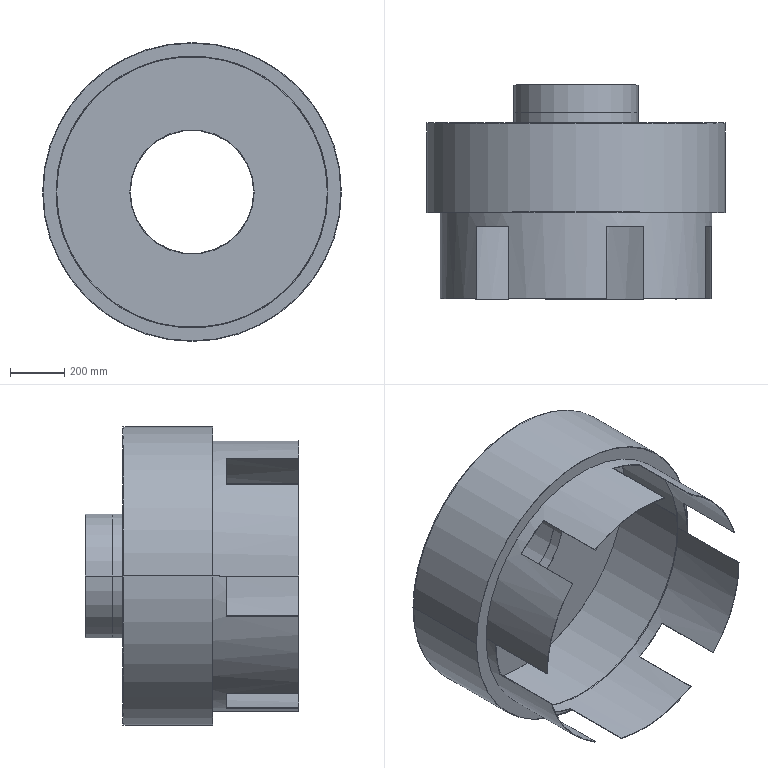Part | SolidWorks | features ICE 2, CirPattern 1, Revolution 1, Shell 1, WeldmentFeature 1 | 1 solid | 44 faces | box 1104 x 790 x 1104 mm | volume 5979369 mm3 | plane 30 | cylinder 14 | commonest cylinder face diameters 456 x2 458 x2 460 x2 1000 x2 1004 x2 1100 x2
STEP:
#1=CARTESIAN_POINT('',(229.,689.,0.));
#2=VERTEX_POINT('',#1);
#3=CARTESIAN_POINT('',(-229.,689.,0.));
#4=VERTEX_POINT('',#3);
#5=CARTESIAN_POINT('',(0.,689.,0.));
#6=DIRECTION('',(0.,1.,0.));
#7=DIRECTION('',(-1.,0.,0.));
#8=AXIS2_PLACEMENT_3D('',#5,#6,#7);
#9=CIRCLE('',#8,229.);
#10=EDGE_CURVE('',#2,#4,#9,.T.);
#11=ORIENTED_EDGE('',*,*,#10,.F.);
#12=CARTESIAN_POINT('',(229.,790.,0.));
#13=VERTEX_POINT('',#12);
#14=CARTESIAN_POINT('',(229.,689.,0.));
#15=DIRECTION('',(0.,1.,0.));
#16=VECTOR('',#15,1000.);
#17=LINE('',#14,#16);
#18=EDGE_CURVE('',#2,#13,#17,.T.);
#19=ORIENTED_EDGE('',*,*,#18,.T.);
#20=CARTESIAN_POINT('',(-229.,790.,0.));
#21=VERTEX_POINT('',#20);
#22=CARTESIAN_POINT('',(0.,790.,0.));
#23=DIRECTION('',(0.,1.,0.));
#24=DIRECTION('',(-1.,0.,0.));
#25=AXIS2_PLACEMENT_3D('',#22,#23,#24);
#26=CIRCLE('',#25,229.);
#27=EDGE_CURVE('',#13,#21,#26,.T.);
#28=ORIENTED_EDGE('',*,*,#27,.T.);
#29=CARTESIAN_POINT('',(-229.,689.,0.));
#30=DIRECTION('',(0.,1.,0.));
#31=VECTOR('',#30,1000.);
#32=LINE('',#29,#31);
#33=EDGE_CURVE('',#4,#21,#32,.T.);
#34=ORIENTED_EDGE('',*,*,#33,.F.);
#35=EDGE_LOOP('',(#11,#19,#28,#34));
#36=FACE_OUTER_BOUND('',#35,.T.);
#37=CARTESIAN_POINT('',(0.,689.,0.));
#38=DIRECTION('',(0.,1.,0.));
#39=DIRECTION('',(-1.,0.,0.));
#40=AXIS2_PLACEMENT_3D('',#37,#38,#39);
#41=CYLINDRICAL_SURFACE('',#40,229.);
#42=ADVANCED_FACE('',(#36),#41,.F.);
#43=CARTESIAN_POINT('',(-550.,648.,0.));
#44=VERTEX_POINT('',#43);
#45=CARTESIAN_POINT('',(550.,648.,0.));
#46=VERTEX_POINT('',#45);
#47=CARTESIAN_POINT('',(0.,648.,0.));
#48=DIRECTION('',(0.,-1.,0.));
#49=DIRECTION('',(-1.,0.,0.));
#50=AXIS2_PLACEMENT_3D('',#47,#48,#49);
#51=CIRCLE('',#50,550.);
#52=EDGE_CURVE('',#44,#46,#51,.T.);
#53=ORIENTED_EDGE('',*,*,#52,.F.);
#54=CARTESIAN_POINT('',(-550.,320.,0.));
#55=VERTEX_POINT('',#54);
#56=CARTESIAN_POINT('',(-550.,0.,0.));
#57=DIRECTION('',(0.,-1.,0.));
#58=VECTOR('',#57,1000.);
#59=LINE('',#56,#58);
#60=EDGE_CURVE('',#44,#55,#59,.T.);
#61=ORIENTED_EDGE('',*,*,#60,.T.);
#62=CARTESIAN_POINT('',(550.,320.,0.));
#63=VERTEX_POINT('',#62);
#64=CARTESIAN_POINT('',(0.,320.,0.));
#65=DIRECTION('',(0.,-1.,0.));
#66=DIRECTION('',(1.,0.,0.));
#67=AXIS2_PLACEMENT_3D('',#64,#65,#66);
#68=CIRCLE('',#67,550.);
#69=EDGE_CURVE('',#55,#63,#68,.T.);
#70=ORIENTED_EDGE('',*,*,#69,.T.);
#71=CARTESIAN_POINT('',(550.,0.,0.));
#72=DIRECTION('',(0.,-1.,0.));
#73=VECTOR('',#72,1000.);
#74=LINE('',#71,#73);
#75=EDGE_CURVE('',#46,#63,#74,.T.);
#76=ORIENTED_EDGE('',*,*,#75,.F.);
#77=EDGE_LOOP('',(#53,#61,#70,#76));
#78=FACE_OUTER_BOUND('',#77,.T.);
#79=CARTESIAN_POINT('',(0.,0.,0.));
#80=DIRECTION('',(0.,-1.,0.));
#81=DIRECTION('',(1.,0.,0.));
#82=AXIS2_PLACEMENT_3D('',#79,#80,#81);
#83=CYLINDRICAL_SURFACE('',#82,550.);
#84=ADVANCED_FACE('',(#78),#83,.F.);
#85=CARTESIAN_POINT('',(552.,650.,0.));
#86=VERTEX_POINT('',#85);
#87=CARTESIAN_POINT('',(-552.,650.,0.));
#88=VERTEX_POINT('',#87);
#89=CARTESIAN_POINT('',(0.,650.,0.));
#90=DIRECTION('',(0.,-1.,0.));
#91=DIRECTION('',(1.,0.,0.));
#92=AXIS2_PLACEMENT_3D('',#89,#90,#91);
#93=CIRCLE('',#92,552.);
#94=EDGE_CURVE('',#86,#88,#93,.T.);
#95=ORIENTED_EDGE('',*,*,#94,.T.);
#96=CARTESIAN_POINT('',(-552.,318.,0.));
#97=VERTEX_POINT('',#96);
#98=CARTESIAN_POINT('',(-552.,0.,0.));
#99=DIRECTION('',(0.,-1.,0.));
#100=VECTOR('',#99,1000.);
#101=LINE('',#98,#100);
#102=EDGE_CURVE('',#88,#97,#101,.T.);
#103=ORIENTED_EDGE('',*,*,#102,.T.);
#104=CARTESIAN_POINT('',(552.,318.,0.));
#105=VERTEX_POINT('',#104);
#106=CARTESIAN_POINT('',(0.,318.,0.));
#107=DIRECTION('',(0.,-1.,0.));
#108=DIRECTION('',(1.,0.,0.));
#109=AXIS2_PLACEMENT_3D('',#106,#107,#108);
#110=CIRCLE('',#109,552.);
#111=EDGE_CURVE('',#105,#97,#110,.T.);
#112=ORIENTED_EDGE('',*,*,#111,.F.);
#113=CARTESIAN_POINT('',(552.,0.,0.));
#114=DIRECTION('',(0.,-1.,0.));
#115=VECTOR('',#114,1000.);
#116=LINE('',#113,#115);
#117=EDGE_CURVE('',#86,#105,#116,.T.);
#118=ORIENTED_EDGE('',*,*,#117,.F.);
#119=EDGE_LOOP('',(#95,#103,#112,#118));
#120=FACE_OUTER_BOUND('',#119,.T.);
#121=CARTESIAN_POINT('',(0.,0.,0.));
#122=DIRECTION('',(0.,-1.,0.));
#123=DIRECTION('',(1.,0.,0.));
#124=AXIS2_PLACEMENT_3D('',#121,#122,#123);
#125=CYLINDRICAL_SURFACE('',#124,552.);
#126=ADVANCED_FACE('',(#120),#125,.T.);
#127=CARTESIAN_POINT('',(230.,790.,0.));
#128=VERTEX_POINT('',#127);
#129=CARTESIAN_POINT('',(-230.,790.,0.));
#130=VERTEX_POINT('',#129);
#131=CARTESIAN_POINT('',(0.,790.,0.));
#132=DIRECTION('',(0.,-1.,0.));
#133=DIRECTION('',(1.,0.,0.));
#134=AXIS2_PLACEMENT_3D('',#131,#132,#133);
#135=CIRCLE('',#134,230.);
#136=EDGE_CURVE('',#128,#130,#135,.T.);
#137=ORIENTED_EDGE('',*,*,#136,.T.);
#138=CARTESIAN_POINT('',(-230.,650.,0.));
#139=VERTEX_POINT('',#138);
#140=CARTESIAN_POINT('',(-230.,0.,0.));
#141=DIRECTION('',(0.,-1.,0.));
#142=VECTOR('',#141,1000.);
#143=LINE('',#140,#142);
#144=EDGE_CURVE('',#130,#139,#143,.T.);
#145=ORIENTED_EDGE('',*,*,#144,.T.);
#146=CARTESIAN_POINT('',(230.,650.,0.));
#147=VERTEX_POINT('',#146);
#148=CARTESIAN_POINT('',(0.,650.,0.));
#149=DIRECTION('',(0.,-1.,0.));
#150=DIRECTION('',(1.,0.,0.));
#151=AXIS2_PLACEMENT_3D('',#148,#149,#150);
#152=CIRCLE('',#151,230.);
#153=EDGE_CURVE('',#147,#139,#152,.T.);
#154=ORIENTED_EDGE('',*,*,#153,.F.);
#155=CARTESIAN_POINT('',(230.,0.,0.));
#156=DIRECTION('',(0.,-1.,0.));
#157=VECTOR('',#156,1000.);
#158=LINE('',#155,#157);
#159=EDGE_CURVE('',#128,#147,#158,.T.);
#160=ORIENTED_EDGE('',*,*,#159,.F.);
#161=EDGE_LOOP('',(#137,#145,#154,#160));
#162=FACE_OUTER_BOUND('',#161,.T.);
#163=CARTESIAN_POINT('',(0.,0.,0.));
#164=DIRECTION('',(0.,-1.,0.));
#165=DIRECTION('',(1.,0.,0.));
#166=AXIS2_PLACEMENT_3D('',#163,#164,#165);
#167=CYLINDRICAL_SURFACE('',#166,230.);
#168=ADVANCED_FACE('',(#162),#167,.T.);
#169=CARTESIAN_POINT('',(-228.,689.,0.));
#170=VERTEX_POINT('',#169);
#171=CARTESIAN_POINT('',(228.,689.,0.));
#172=VERTEX_POINT('',#171);
#173=CARTESIAN_POINT('',(0.,689.,0.));
#174=DIRECTION('',(0.,-1.,0.));
#175=DIRECTION('',(-1.,0.,0.));
#176=AXIS2_PLACEMENT_3D('',#173,#174,#175);
#177=CIRCLE('',#176,228.);
#178=EDGE_CURVE('',#170,#172,#177,.T.);
#179=ORIENTED_EDGE('',*,*,#178,.F.);
#180=CARTESIAN_POINT('',(-228.,648.,0.));
#181=VERTEX_POINT('',#180);
#182=CARTESIAN_POINT('',(-228.,0.,0.));
#183=DIRECTION('',(0.,-1.,0.));
#184=VECTOR('',#183,1000.);
#185=LINE('',#182,#184);
#186=EDGE_CURVE('',#170,#181,#185,.T.);
#187=ORIENTED_EDGE('',*,*,#186,.T.);
#188=CARTESIAN_POINT('',(228.,648.,0.));
#189=VERTEX_POINT('',#188);
#190=CARTESIAN_POINT('',(0.,648.,0.));
#191=DIRECTION('',(0.,-1.,0.));
#192=DIRECTION('',(-1.,0.,0.));
#193=AXIS2_PLACEMENT_3D('',#190,#191,#192);
#194=CIRCLE('',#193,228.);
#195=EDGE_CURVE('',#181,#189,#194,.T.);
#196=ORIENTED_EDGE('',*,*,#195,.T.);
#197=CARTESIAN_POINT('',(228.,0.,0.));
#198=DIRECTION('',(0.,-1.,0.));
#199=VECTOR('',#198,1000.);
#200=LINE('',#197,#199);
#201=EDGE_CURVE('',#172,#189,#200,.T.);
#202=ORIENTED_EDGE('',*,*,#201,.F.);
#203=EDGE_LOOP('',(#179,#187,#196,#202));
#204=FACE_OUTER_BOUND('',#203,.T.);
#205=CARTESIAN_POINT('',(0.,0.,0.));
#206=DIRECTION('',(0.,-1.,0.));
#207=DIRECTION('',(1.,0.,0.));
#208=AXIS2_PLACEMENT_3D('',#205,#206,#207);
#209=CYLINDRICAL_SURFACE('',#208,228.);
#210=ADVANCED_FACE('',(#204),#209,.F.);
#211=CARTESIAN_POINT('',(-500.,320.,0.));
#212=VERTEX_POINT('',#211);
#213=CARTESIAN_POINT('',(500.,320.,0.));
#214=VERTEX_POINT('',#213);
#215=CARTESIAN_POINT('',(0.,320.,0.));
#216=DIRECTION('',(0.,-1.,0.));
#217=DIRECTION('',(1.,0.,0.));
#218=AXIS2_PLACEMENT_3D('',#215,#216,#217);
#219=CIRCLE('',#218,500.);
#220=EDGE_CURVE('',#212,#214,#219,.T.);
#221=ORIENTED_EDGE('',*,*,#220,.F.);
#222=CARTESIAN_POINT('',(-500.,268.,0.));
#223=VERTEX_POINT('',#222);
#224=CARTESIAN_POINT('',(-500.,0.,0.));
#225=DIRECTION('',(0.,-1.,0.));
#226=VECTOR('',#225,1000.);
#227=LINE('',#224,#226);
#228=EDGE_CURVE('',#212,#223,#227,.T.);
#229=ORIENTED_EDGE('',*,*,#228,.T.);
#230=CARTESIAN_POINT('',(-477.679,268.,-147.726));
#231=VERTEX_POINT('',#230);
#232=CARTESIAN_POINT('',(0.,268.,0.));
#233=DIRECTION('',(0.,1.,0.));
#234=DIRECTION('',(1.,0.,0.));
#235=AXIS2_PLACEMENT_3D('',#232,#233,#234);
#236=CIRCLE('',#235,500.);
#237=EDGE_CURVE('',#231,#223,#236,.T.);
#238=ORIENTED_EDGE('',*,*,#237,.F.);
#239=CARTESIAN_POINT('',(-477.679,0.,-147.726));
#240=VERTEX_POINT('',#239);
#241=CARTESIAN_POINT('',(-477.679,0.,-147.726));
#242=DIRECTION('',(0.,1.,0.));
#243=VECTOR('',#242,1000.);
#244=LINE('',#241,#243);
#245=EDGE_CURVE('',#240,#231,#244,.T.);
#246=ORIENTED_EDGE('',*,*,#245,.F.);
#247=CARTESIAN_POINT('',(-250.,0.,-433.013));
#248=VERTEX_POINT('',#247);
#249=CARTESIAN_POINT('',(0.,0.,0.));
#250=DIRECTION('',(0.,-1.,0.));
#251=DIRECTION('',(1.,0.,0.));
#252=AXIS2_PLACEMENT_3D('',#249,#250,#251);
#253=CIRCLE('',#252,500.);
#254=EDGE_CURVE('',#240,#248,#253,.T.);
#255=ORIENTED_EDGE('',*,*,#254,.T.);
#256=CARTESIAN_POINT('',(-250.,268.,-433.013));
#257=VERTEX_POINT('',#256);
#258=CARTESIAN_POINT('',(-250.,0.,-433.013));
#259=DIRECTION('',(0.,-1.,0.));
#260=VECTOR('',#259,1000.);
#261=LINE('',#258,#260);
#262=EDGE_CURVE('',#257,#248,#261,.T.);
#263=ORIENTED_EDGE('',*,*,#262,.F.);
#264=CARTESIAN_POINT('',(-110.905,268.,-487.545));
#265=VERTEX_POINT('',#264);
#266=CARTESIAN_POINT('',(0.,268.,0.));
#267=DIRECTION('',(0.,1.,0.));
#268=DIRECTION('',(1.,0.,0.));
#269=AXIS2_PLACEMENT_3D('',#266,#267,#268);
#270=CIRCLE('',#269,500.);
#271=EDGE_CURVE('',#265,#257,#270,.T.);
#272=ORIENTED_EDGE('',*,*,#271,.F.);
#273=CARTESIAN_POINT('',(-110.905,0.,-487.545));
#274=VERTEX_POINT('',#273);
#275=CARTESIAN_POINT('',(-110.905,0.,-487.545));
#276=DIRECTION('',(0.,1.,0.));
#277=VECTOR('',#276,1000.);
#278=LINE('',#275,#277);
#279=EDGE_CURVE('',#274,#265,#278,.T.);
#280=ORIENTED_EDGE('',*,*,#279,.F.);
#281=CARTESIAN_POINT('',(250.,0.,-433.013));
#282=VERTEX_POINT('',#281);
#283=CARTESIAN_POINT('',(0.,0.,0.));
#284=DIRECTION('',(0.,-1.,0.));
#285=DIRECTION('',(1.,0.,0.));
#286=AXIS2_PLACEMENT_3D('',#283,#284,#285);
#287=CIRCLE('',#286,500.);
#288=EDGE_CURVE('',#274,#282,#287,.T.);
#289=ORIENTED_EDGE('',*,*,#288,.T.);
#290=CARTESIAN_POINT('',(250.,268.,-433.013));
#291=VERTEX_POINT('',#290);
#292=CARTESIAN_POINT('',(250.,0.,-433.013));
#293=DIRECTION('',(0.,-1.,0.));
#294=VECTOR('',#293,1000.);
#295=LINE('',#292,#294);
#296=EDGE_CURVE('',#291,#282,#295,.T.);
#297=ORIENTED_EDGE('',*,*,#296,.F.);
#298=CARTESIAN_POINT('',(366.774,268.,-339.819));
#299=VERTEX_POINT('',#298);
#300=CARTESIAN_POINT('',(0.,268.,0.));
#301=DIRECTION('',(0.,1.,0.));
#302=DIRECTION('',(1.,0.,0.));
#303=AXIS2_PLACEMENT_3D('',#300,#301,#302);
#304=CIRCLE('',#303,500.);
#305=EDGE_CURVE('',#299,#291,#304,.T.);
#306=ORIENTED_EDGE('',*,*,#305,.F.);
#307=CARTESIAN_POINT('',(366.774,0.,-339.819));
#308=VERTEX_POINT('',#307);
#309=CARTESIAN_POINT('',(366.774,0.,-339.819));
#310=DIRECTION('',(0.,1.,0.));
#311=VECTOR('',#310,1000.);
#312=LINE('',#309,#311);
#313=EDGE_CURVE('',#308,#299,#312,.T.);
#314=ORIENTED_EDGE('',*,*,#313,.F.);
#315=CARTESIAN_POINT('',(500.,0.,0.));
#316=VERTEX_POINT('',#315);
#317=CARTESIAN_POINT('',(0.,0.,0.));
#318=DIRECTION('',(0.,-1.,0.));
#319=DIRECTION('',(1.,0.,0.));
#320=AXIS2_PLACEMENT_3D('',#317,#318,#319);
#321=CIRCLE('',#320,500.);
#322=EDGE_CURVE('',#308,#316,#321,.T.);
#323=ORIENTED_EDGE('',*,*,#322,.T.);
#324=CARTESIAN_POINT('',(500.,268.,0.));
#325=VERTEX_POINT('',#324);
#326=CARTESIAN_POINT('',(500.,0.,0.));
#327=DIRECTION('',(0.,-1.,0.));
#328=VECTOR('',#327,1000.);
#329=LINE('',#326,#328);
#330=EDGE_CURVE('',#325,#316,#329,.T.);
#331=ORIENTED_EDGE('',*,*,#330,.F.);
#332=CARTESIAN_POINT('',(500.,0.,0.));
#333=DIRECTION('',(0.,-1.,0.));
#334=VECTOR('',#333,1000.);
#335=LINE('',#332,#334);
#336=EDGE_CURVE('',#214,#325,#335,.T.);
#337=ORIENTED_EDGE('',*,*,#336,.F.);
#338=EDGE_LOOP('',(#221,#229,#238,#246,#255,#263,#272,#280,#289,#297,#306,#314,#323,#331,#337));
#339=FACE_OUTER_BOUND('',#338,.T.);
#340=CARTESIAN_POINT('',(0.,0.,0.));
#341=DIRECTION('',(0.,-1.,0.));
#342=DIRECTION('',(1.,0.,0.));
#343=AXIS2_PLACEMENT_3D('',#340,#341,#342);
#344=CYLINDRICAL_SURFACE('',#343,500.);
#345=ADVANCED_FACE('',(#339),#344,.F.);
#346=CARTESIAN_POINT('',(502.,318.,0.));
#347=VERTEX_POINT('',#346);
#348=CARTESIAN_POINT('',(-502.,318.,0.));
#349=VERTEX_POINT('',#348);
#350=CARTESIAN_POINT('',(0.,318.,0.));
#351=DIRECTION('',(0.,-1.,0.));
#352=DIRECTION('',(1.,0.,0.));
#353=AXIS2_PLACEMENT_3D('',#350,#351,#352);
#354=CIRCLE('',#353,502.);
#355=EDGE_CURVE('',#347,#349,#354,.T.);
#356=ORIENTED_EDGE('',*,*,#355,.T.);
#357=CARTESIAN_POINT('',(-502.,268.,0.));
#358=VERTEX_POINT('',#357);
#359=CARTESIAN_POINT('',(-502.,0.,0.));
#360=DIRECTION('',(0.,-1.,0.));
#361=VECTOR('',#360,1000.);
#362=LINE('',#359,#361);
#363=EDGE_CURVE('',#349,#358,#362,.T.);
#364=ORIENTED_EDGE('',*,*,#363,.T.);
#365=CARTESIAN_POINT('',(-502.,0.,0.));
#366=VERTEX_POINT('',#365);
#367=CARTESIAN_POINT('',(-502.,0.,0.));
#368=DIRECTION('',(0.,-1.,0.));
#369=VECTOR('',#368,1000.);
#370=LINE('',#367,#369);
#371=EDGE_CURVE('',#358,#366,#370,.T.);
#372=ORIENTED_EDGE('',*,*,#371,.T.);
#373=CARTESIAN_POINT('',(-368.241,0.,341.179));
#374=VERTEX_POINT('',#373);
#375=CARTESIAN_POINT('',(0.,0.,0.));
#376=DIRECTION('',(0.,-1.,0.));
#377=DIRECTION('',(1.,0.,0.));
#378=AXIS2_PLACEMENT_3D('',#375,#376,#377);
#379=CIRCLE('',#378,502.);
#380=EDGE_CURVE('',#374,#366,#379,.T.);
#381=ORIENTED_EDGE('',*,*,#380,.F.);
#382=CARTESIAN_POINT('',(-368.241,268.,341.179));
#383=VERTEX_POINT('',#382);
#384=CARTESIAN_POINT('',(-368.241,0.,341.179));
#385=DIRECTION('',(0.,1.,0.));
#386=VECTOR('',#385,1000.);
#387=LINE('',#384,#386);
#388=EDGE_CURVE('',#374,#383,#387,.T.);
#389=ORIENTED_EDGE('',*,*,#388,.T.);
#390=CARTESIAN_POINT('',(-251.,268.,434.745));
#391=VERTEX_POINT('',#390);
#392=CARTESIAN_POINT('',(0.,268.,0.));
#393=DIRECTION('',(0.,1.,0.));
#394=DIRECTION('',(1.,0.,0.));
#395=AXIS2_PLACEMENT_3D('',#392,#393,#394);
#396=CIRCLE('',#395,502.);
#397=EDGE_CURVE('',#383,#391,#396,.T.);
#398=ORIENTED_EDGE('',*,*,#397,.T.);
#399=CARTESIAN_POINT('',(-251.,0.,434.745));
#400=VERTEX_POINT('',#399);
#401=CARTESIAN_POINT('',(-251.,0.,434.745));
#402=DIRECTION('',(0.,-1.,0.));
#403=VECTOR('',#402,1000.);
#404=LINE('',#401,#403);
#405=EDGE_CURVE('',#391,#400,#404,.T.);
#406=ORIENTED_EDGE('',*,*,#405,.T.);
#407=CARTESIAN_POINT('',(111.349,0.,489.495));
#408=VERTEX_POINT('',#407);
#409=CARTESIAN_POINT('',(0.,0.,0.));
#410=DIRECTION('',(0.,-1.,0.));
#411=DIRECTION('',(1.,0.,0.));
#412=AXIS2_PLACEMENT_3D('',#409,#410,#411);
#413=CIRCLE('',#412,502.);
#414=EDGE_CURVE('',#408,#400,#413,.T.);
#415=ORIENTED_EDGE('',*,*,#414,.F.);
#416=CARTESIAN_POINT('',(111.349,268.,489.495));
#417=VERTEX_POINT('',#416);
#418=CARTESIAN_POINT('',(111.349,0.,489.495));
#419=DIRECTION('',(0.,1.,0.));
#420=VECTOR('',#419,1000.);
#421=LINE('',#418,#420);
#422=EDGE_CURVE('',#408,#417,#421,.T.);
#423=ORIENTED_EDGE('',*,*,#422,.T.);
#424=CARTESIAN_POINT('',(251.,268.,434.745));
#425=VERTEX_POINT('',#424);
#426=CARTESIAN_POINT('',(0.,268.,0.));
#427=DIRECTION('',(0.,1.,0.));
#428=DIRECTION('',(1.,0.,0.));
#429=AXIS2_PLACEMENT_3D('',#426,#427,#428);
#430=CIRCLE('',#429,502.);
#431=EDGE_CURVE('',#417,#425,#430,.T.);
#432=ORIENTED_EDGE('',*,*,#431,.T.);
#433=CARTESIAN_POINT('',(251.,0.,434.745));
#434=VERTEX_POINT('',#433);
#435=CARTESIAN_POINT('',(251.,0.,434.745));
#436=DIRECTION('',(0.,-1.,0.));
#437=VECTOR('',#436,1000.);
#438=LINE('',#435,#437);
#439=EDGE_CURVE('',#425,#434,#438,.T.);
#440=ORIENTED_EDGE('',*,*,#439,.T.);
#441=CARTESIAN_POINT('',(479.59,0.,148.316));
#442=VERTEX_POINT('',#441);
#443=CARTESIAN_POINT('',(0.,0.,0.));
#444=DIRECTION('',(0.,-1.,0.));
#445=DIRECTION('',(1.,0.,0.));
#446=AXIS2_PLACEMENT_3D('',#443,#444,#445);
#447=CIRCLE('',#446,502.);
#448=EDGE_CURVE('',#442,#434,#447,.T.);
#449=ORIENTED_EDGE('',*,*,#448,.F.);
#450=CARTESIAN_POINT('',(479.59,268.,148.316));
#451=VERTEX_POINT('',#450);
#452=CARTESIAN_POINT('',(479.59,0.,148.316));
#453=DIRECTION('',(0.,1.,0.));
#454=VECTOR('',#453,1000.);
#455=LINE('',#452,#454);
#456=EDGE_CURVE('',#442,#451,#455,.T.);
#457=ORIENTED_EDGE('',*,*,#456,.T.);
#458=CARTESIAN_POINT('',(502.,268.,0.));
#459=VERTEX_POINT('',#458);
#460=CARTESIAN_POINT('',(0.,268.,0.));
#461=DIRECTION('',(0.,1.,0.));
#462=DIRECTION('',(1.,0.,0.));
#463=AXIS2_PLACEMENT_3D('',#460,#461,#462);
#464=CIRCLE('',#463,502.);
#465=EDGE_CURVE('',#451,#459,#464,.T.);
#466=ORIENTED_EDGE('',*,*,#465,.T.);
#467=CARTESIAN_POINT('',(502.,0.,0.));
#468=DIRECTION('',(0.,-1.,0.));
#469=VECTOR('',#468,1000.);
#470=LINE('',#467,#469);
#471=EDGE_CURVE('',#347,#459,#470,.T.);
#472=ORIENTED_EDGE('',*,*,#471,.F.);
#473=EDGE_LOOP('',(#356,#364,#372,#381,#389,#398,#406,#415,#423,#432,#440,#449,#457,#466,#472));
#474=FACE_OUTER_BOUND('',#473,.T.);
#475=CARTESIAN_POINT('',(0.,0.,0.));
#476=DIRECTION('',(0.,-1.,0.));
#477=DIRECTION('',(1.,0.,0.));
#478=AXIS2_PLACEMENT_3D('',#475,#476,#477);
#479=CYLINDRICAL_SURFACE('',#478,502.);
#480=ADVANCED_FACE('',(#474),#479,.T.);
#481=ORIENTED_EDGE('',*,*,#448,.T.);
#482=CARTESIAN_POINT('',(250.,0.,433.013));
#483=VERTEX_POINT('',#482);
#484=CARTESIAN_POINT('',(0.,0.,0.));
#485=DIRECTION('',(-0.5,0.,-0.866));
#486=VECTOR('',#485,1000.);
#487=LINE('',#484,#486);
#488=EDGE_CURVE('',#434,#483,#487,.T.);
#489=ORIENTED_EDGE('',*,*,#488,.T.);
#490=CARTESIAN_POINT('',(477.679,0.,147.726));
#491=VERTEX_POINT('',#490);
#492=CARTESIAN_POINT('',(0.,0.,0.));
#493=DIRECTION('',(0.,-1.,0.));
#494=DIRECTION('',(1.,0.,0.));
#495=AXIS2_PLACEMENT_3D('',#492,#493,#494);
#496=CIRCLE('',#495,500.);
#497=EDGE_CURVE('',#491,#483,#496,.T.);
#498=ORIENTED_EDGE('',*,*,#497,.F.);
#499=CARTESIAN_POINT('',(0.,0.,0.));
#500=DIRECTION('',(0.9554,0.,0.2955));
#501=VECTOR('',#500,1000.);
#502=LINE('',#499,#501);
#503=EDGE_CURVE('',#491,#442,#502,.T.);
#504=ORIENTED_EDGE('',*,*,#503,.T.);
#505=EDGE_LOOP('',(#481,#489,#498,#504));
#506=FACE_OUTER_BOUND('',#505,.T.);
#507=CARTESIAN_POINT('',(502.,0.,0.));
#508=DIRECTION('',(0.,-1.,0.));
#509=DIRECTION('',(1.,0.,0.));
#510=AXIS2_PLACEMENT_3D('',#507,#508,#509);
#511=PLANE('',#510);
#512=ADVANCED_FACE('',(#506),#511,.T.);
#513=CARTESIAN_POINT('',(110.905,0.,487.545));
#514=VERTEX_POINT('',#513);
#515=CARTESIAN_POINT('',(-250.,0.,433.013));
#516=VERTEX_POINT('',#515);
#517=CARTESIAN_POINT('',(0.,0.,0.));
#518=DIRECTION('',(0.,-1.,0.));
#519=DIRECTION('',(1.,0.,0.));
#520=AXIS2_PLACEMENT_3D('',#517,#518,#519);
#521=CIRCLE('',#520,500.);
#522=EDGE_CURVE('',#514,#516,#521,.T.);
#523=ORIENTED_EDGE('',*,*,#522,.F.);
#524=CARTESIAN_POINT('',(0.,0.,0.));
#525=DIRECTION('',(0.2218,0.,0.9751));
#526=VECTOR('',#525,1000.);
#527=LINE('',#524,#526);
#528=EDGE_CURVE('',#514,#408,#527,.T.);
#529=ORIENTED_EDGE('',*,*,#528,.T.);
#530=ORIENTED_EDGE('',*,*,#414,.T.);
#531=CARTESIAN_POINT('',(0.,0.,0.));
#532=DIRECTION('',(0.5,0.,-0.866));
#533=VECTOR('',#532,1000.);
#534=LINE('',#531,#533);
#535=EDGE_CURVE('',#400,#516,#534,.T.);
#536=ORIENTED_EDGE('',*,*,#535,.T.);
#537=EDGE_LOOP('',(#523,#529,#530,#536));
#538=FACE_OUTER_BOUND('',#537,.T.);
#539=CARTESIAN_POINT('',(502.,0.,0.));
#540=DIRECTION('',(0.,-1.,0.));
#541=DIRECTION('',(1.,0.,0.));
#542=AXIS2_PLACEMENT_3D('',#539,#540,#541);
#543=PLANE('',#542);
#544=ADVANCED_FACE('',(#538),#543,.T.);
#545=ORIENTED_EDGE('',*,*,#363,.F.);
#546=CARTESIAN_POINT('',(0.,318.,0.));
#547=DIRECTION('',(0.,-1.,0.));
#548=DIRECTION('',(1.,0.,0.));
#549=AXIS2_PLACEMENT_3D('',#546,#547,#548);
#550=CIRCLE('',#549,502.);
#551=EDGE_CURVE('',#349,#347,#550,.T.);
#552=ORIENTED_EDGE('',*,*,#551,.T.);
#553=ORIENTED_EDGE('',*,*,#471,.T.);
#554=CARTESIAN_POINT('',(502.,0.,0.));
#555=VERTEX_POINT('',#554);
#556=CARTESIAN_POINT('',(502.,0.,0.));
#557=DIRECTION('',(0.,-1.,0.));
#558=VECTOR('',#557,1000.);
#559=LINE('',#556,#558);
#560=EDGE_CURVE('',#459,#555,#559,.T.);
#561=ORIENTED_EDGE('',*,*,#560,.T.);
#562=CARTESIAN_POINT('',(368.241,0.,-341.179));
#563=VERTEX_POINT('',#562);
#564=CARTESIAN_POINT('',(0.,0.,0.));
#565=DIRECTION('',(0.,-1.,0.));
#566=DIRECTION('',(1.,0.,0.));
#567=AXIS2_PLACEMENT_3D('',#564,#565,#566);
#568=CIRCLE('',#567,502.);
#569=EDGE_CURVE('',#563,#555,#568,.T.);
#570=ORIENTED_EDGE('',*,*,#569,.F.);
#571=CARTESIAN_POINT('',(368.241,268.,-341.179));
#572=VERTEX_POINT('',#571);
#573=CARTESIAN_POINT('',(368.241,0.,-341.179));
#574=DIRECTION('',(0.,1.,0.));
#575=VECTOR('',#574,1000.);
#576=LINE('',#573,#575);
#577=EDGE_CURVE('',#563,#572,#576,.T.);
#578=ORIENTED_EDGE('',*,*,#577,.T.);
#579=CARTESIAN_POINT('',(251.,268.,-434.745));
#580=VERTEX_POINT('',#579);
#581=CARTESIAN_POINT('',(0.,268.,0.));
#582=DIRECTION('',(0.,1.,0.));
#583=DIRECTION('',(1.,0.,0.));
#584=AXIS2_PLACEMENT_3D('',#581,#582,#583);
#585=CIRCLE('',#584,502.);
#586=EDGE_CURVE('',#572,#580,#585,.T.);
#587=ORIENTED_EDGE('',*,*,#586,.T.);
#588=CARTESIAN_POINT('',(251.,0.,-434.745));
#589=VERTEX_POINT('',#588);
#590=CARTESIAN_POINT('',(251.,0.,-434.745));
#591=DIRECTION('',(0.,-1.,0.));
#592=VECTOR('',#591,1000.);
#593=LINE('',#590,#592);
#594=EDGE_CURVE('',#580,#589,#593,.T.);
#595=ORIENTED_EDGE('',*,*,#594,.T.);
#596=CARTESIAN_POINT('',(-111.349,0.,-489.495));
#597=VERTEX_POINT('',#596);
#598=CARTESIAN_POINT('',(0.,0.,0.));
#599=DIRECTION('',(0.,-1.,0.));
#600=DIRECTION('',(1.,0.,0.));
#601=AXIS2_PLACEMENT_3D('',#598,#599,#600);
#602=CIRCLE('',#601,502.);
#603=EDGE_CURVE('',#597,#589,#602,.T.);
#604=ORIENTED_EDGE('',*,*,#603,.F.);
#605=CARTESIAN_POINT('',(-111.349,268.,-489.495));
#606=VERTEX_POINT('',#605);
#607=CARTESIAN_POINT('',(-111.349,0.,-489.495));
#608=DIRECTION('',(0.,1.,0.));
#609=VECTOR('',#608,1000.);
#610=LINE('',#607,#609);
#611=EDGE_CURVE('',#597,#606,#610,.T.);
#612=ORIENTED_EDGE('',*,*,#611,.T.);
#613=CARTESIAN_POINT('',(-251.,268.,-434.745));
#614=VERTEX_POINT('',#613);
#615=CARTESIAN_POINT('',(0.,268.,0.));
#616=DIRECTION('',(0.,1.,0.));
#617=DIRECTION('',(1.,0.,0.));
#618=AXIS2_PLACEMENT_3D('',#615,#616,#617);
#619=CIRCLE('',#618,502.);
#620=EDGE_CURVE('',#606,#614,#619,.T.);
#621=ORIENTED_EDGE('',*,*,#620,.T.);
#622=CARTESIAN_POINT('',(-251.,0.,-434.745));
#623=VERTEX_POINT('',#622);
#624=CARTESIAN_POINT('',(-251.,0.,-434.745));
#625=DIRECTION('',(0.,-1.,0.));
#626=VECTOR('',#625,1000.);
#627=LINE('',#624,#626);
#628=EDGE_CURVE('',#614,#623,#627,.T.);
#629=ORIENTED_EDGE('',*,*,#628,.T.);
#630=CARTESIAN_POINT('',(-479.59,0.,-148.316));
#631=VERTEX_POINT('',#630);
#632=CARTESIAN_POINT('',(0.,0.,0.));
#633=DIRECTION('',(0.,-1.,0.));
#634=DIRECTION('',(1.,0.,0.));
#635=AXIS2_PLACEMENT_3D('',#632,#633,#634);
#636=CIRCLE('',#635,502.);
#637=EDGE_CURVE('',#631,#623,#636,.T.);
#638=ORIENTED_EDGE('',*,*,#637,.F.);
#639=CARTESIAN_POINT('',(-479.59,268.,-148.316));
#640=VERTEX_POINT('',#639);
#641=CARTESIAN_POINT('',(-479.59,0.,-148.316));
#642=DIRECTION('',(0.,1.,0.));
#643=VECTOR('',#642,1000.);
#644=LINE('',#641,#643);
#645=EDGE_CURVE('',#631,#640,#644,.T.);
#646=ORIENTED_EDGE('',*,*,#645,.T.);
#647=CARTESIAN_POINT('',(0.,268.,0.));
#648=DIRECTION('',(0.,1.,0.));
#649=DIRECTION('',(1.,0.,0.));
#650=AXIS2_PLACEMENT_3D('',#647,#648,#649);
#651=CIRCLE('',#650,502.);
#652=EDGE_CURVE('',#640,#358,#651,.T.);
#653=ORIENTED_EDGE('',*,*,#652,.T.);
#654=EDGE_LOOP('',(#545,#552,#553,#561,#570,#578,#587,#595,#604,#612,#621,#629,#638,#646,#653));
#655=FACE_OUTER_BOUND('',#654,.T.);
#656=CARTESIAN_POINT('',(0.,0.,0.));
#657=DIRECTION('',(0.,-1.,0.));
#658=DIRECTION('',(1.,0.,0.));
#659=AXIS2_PLACEMENT_3D('',#656,#657,#658);
#660=CYLINDRICAL_SURFACE('',#659,502.);
#661=ADVANCED_FACE('',(#655),#660,.T.);
#662=ORIENTED_EDGE('',*,*,#228,.F.);
#663=CARTESIAN_POINT('',(0.,320.,0.));
#664=DIRECTION('',(0.,-1.,0.));
#665=DIRECTION('',(1.,0.,0.));
#666=AXIS2_PLACEMENT_3D('',#663,#664,#665);
#667=CIRCLE('',#666,500.);
#668=EDGE_CURVE('',#214,#212,#667,.T.);
#669=ORIENTED_EDGE('',*,*,#668,.F.);
#670=ORIENTED_EDGE('',*,*,#336,.T.);
#671=CARTESIAN_POINT('',(477.679,268.,147.726));
#672=VERTEX_POINT('',#671);
#673=CARTESIAN_POINT('',(0.,268.,0.));
#674=DIRECTION('',(0.,1.,0.));
#675=DIRECTION('',(1.,0.,0.));
#676=AXIS2_PLACEMENT_3D('',#673,#674,#675);
#677=CIRCLE('',#676,500.);
#678=EDGE_CURVE('',#672,#325,#677,.T.);
#679=ORIENTED_EDGE('',*,*,#678,.F.);
#680=CARTESIAN_POINT('',(477.679,0.,147.726));
#681=DIRECTION('',(0.,1.,0.));
#682=VECTOR('',#681,1000.);
#683=LINE('',#680,#682);
#684=EDGE_CURVE('',#491,#672,#683,.T.);
#685=ORIENTED_EDGE('',*,*,#684,.F.);
#686=ORIENTED_EDGE('',*,*,#497,.T.);
#687=CARTESIAN_POINT('',(250.,268.,433.013));
#688=VERTEX_POINT('',#687);
#689=CARTESIAN_POINT('',(250.,0.,433.013));
#690=DIRECTION('',(0.,-1.,0.));
#691=VECTOR('',#690,1000.);
#692=LINE('',#689,#691);
#693=EDGE_CURVE('',#688,#483,#692,.T.);
#694=ORIENTED_EDGE('',*,*,#693,.F.);
#695=CARTESIAN_POINT('',(110.905,268.,487.545));
#696=VERTEX_POINT('',#695);
#697=CARTESIAN_POINT('',(0.,268.,0.));
#698=DIRECTION('',(0.,1.,0.));
#699=DIRECTION('',(1.,0.,0.));
#700=AXIS2_PLACEMENT_3D('',#697,#698,#699);
#701=CIRCLE('',#700,500.);
#702=EDGE_CURVE('',#696,#688,#701,.T.);
#703=ORIENTED_EDGE('',*,*,#702,.F.);
#704=CARTESIAN_POINT('',(110.905,0.,487.545));
#705=DIRECTION('',(0.,1.,0.));
#706=VECTOR('',#705,1000.);
#707=LINE('',#704,#706);
#708=EDGE_CURVE('',#514,#696,#707,.T.);
#709=ORIENTED_EDGE('',*,*,#708,.F.);
#710=ORIENTED_EDGE('',*,*,#522,.T.);
#711=CARTESIAN_POINT('',(-250.,268.,433.013));
#712=VERTEX_POINT('',#711);
#713=CARTESIAN_POINT('',(-250.,0.,433.013));
#714=DIRECTION('',(0.,-1.,0.));
#715=VECTOR('',#714,1000.);
#716=LINE('',#713,#715);
#717=EDGE_CURVE('',#712,#516,#716,.T.);
#718=ORIENTED_EDGE('',*,*,#717,.F.);
#719=CARTESIAN_POINT('',(-366.774,268.,339.819));
#720=VERTEX_POINT('',#719);
#721=CARTESIAN_POINT('',(0.,268.,0.));
#722=DIRECTION('',(0.,1.,0.));
#723=DIRECTION('',(1.,0.,0.));
#724=AXIS2_PLACEMENT_3D('',#721,#722,#723);
#725=CIRCLE('',#724,500.);
#726=EDGE_CURVE('',#720,#712,#725,.T.);
#727=ORIENTED_EDGE('',*,*,#726,.F.);
#728=CARTESIAN_POINT('',(-366.774,0.,339.819));
#729=VERTEX_POINT('',#728);
#730=CARTESIAN_POINT('',(-366.774,0.,339.819));
#731=DIRECTION('',(0.,1.,0.));
#732=VECTOR('',#731,1000.);
#733=LINE('',#730,#732);
#734=EDGE_CURVE('',#729,#720,#733,.T.);
#735=ORIENTED_EDGE('',*,*,#734,.F.);
#736=CARTESIAN_POINT('',(-500.,0.,0.));
#737=VERTEX_POINT('',#736);
#738=CARTESIAN_POINT('',(0.,0.,0.));
#739=DIRECTION('',(0.,-1.,0.));
#740=DIRECTION('',(1.,0.,0.));
#741=AXIS2_PLACEMENT_3D('',#738,#739,#740);
#742=CIRCLE('',#741,500.);
#743=EDGE_CURVE('',#729,#737,#742,.T.);
#744=ORIENTED_EDGE('',*,*,#743,.T.);
#745=CARTESIAN_POINT('',(-500.,0.,0.));
#746=DIRECTION('',(0.,-1.,0.));
#747=VECTOR('',#746,1000.);
#748=LINE('',#745,#747);
#749=EDGE_CURVE('',#223,#737,#748,.T.);
#750=ORIENTED_EDGE('',*,*,#749,.F.);
#751=EDGE_LOOP('',(#662,#669,#670,#679,#685,#686,#694,#703,#709,#710,#718,#727,#735,#744,#750));
#752=FACE_OUTER_BOUND('',#751,.T.);
#753=CARTESIAN_POINT('',(0.,0.,0.));
#754=DIRECTION('',(0.,-1.,0.));
#755=DIRECTION('',(1.,0.,0.));
#756=AXIS2_PLACEMENT_3D('',#753,#754,#755);
#757=CYLINDRICAL_SURFACE('',#756,500.);
#758=ADVANCED_FACE('',(#752),#757,.F.);
#759=ORIENTED_EDGE('',*,*,#743,.F.);
#760=CARTESIAN_POINT('',(0.,0.,0.));
#761=DIRECTION('',(-0.7335,0.,0.6796));
#762=VECTOR('',#761,1000.);
#763=LINE('',#760,#762);
#764=EDGE_CURVE('',#729,#374,#763,.T.);
#765=ORIENTED_EDGE('',*,*,#764,.T.);
#766=ORIENTED_EDGE('',*,*,#380,.T.);
#767=CARTESIAN_POINT('',(0.,0.,0.));
#768=DIRECTION('',(1.,0.,0.));
#769=VECTOR('',#768,1000.);
#770=LINE('',#767,#769);
#771=EDGE_CURVE('',#366,#737,#770,.T.);
#772=ORIENTED_EDGE('',*,*,#771,.T.);
#773=EDGE_LOOP('',(#759,#765,#766,#772));
#774=FACE_OUTER_BOUND('',#773,.T.);
#775=CARTESIAN_POINT('',(502.,0.,0.));
#776=DIRECTION('',(0.,-1.,0.));
#777=DIRECTION('',(1.,0.,0.));
#778=AXIS2_PLACEMENT_3D('',#775,#776,#777);
#779=PLANE('',#778);
#780=ADVANCED_FACE('',(#774),#779,.T.);
#781=ORIENTED_EDGE('',*,*,#254,.F.);
#782=CARTESIAN_POINT('',(0.,0.,0.));
#783=DIRECTION('',(-0.9554,0.,-0.2955));
#784=VECTOR('',#783,1000.);
#785=LINE('',#782,#784);
#786=EDGE_CURVE('',#240,#631,#785,.T.);
#787=ORIENTED_EDGE('',*,*,#786,.T.);
#788=ORIENTED_EDGE('',*,*,#637,.T.);
#789=CARTESIAN_POINT('',(0.,0.,0.));
#790=DIRECTION('',(0.5,0.,0.866));
#791=VECTOR('',#790,1000.);
#792=LINE('',#789,#791);
#793=EDGE_CURVE('',#623,#248,#792,.T.);
#794=ORIENTED_EDGE('',*,*,#793,.T.);
#795=EDGE_LOOP('',(#781,#787,#788,#794));
#796=FACE_OUTER_BOUND('',#795,.T.);
#797=CARTESIAN_POINT('',(502.,0.,0.));
#798=DIRECTION('',(0.,-1.,0.));
#799=DIRECTION('',(1.,0.,0.));
#800=AXIS2_PLACEMENT_3D('',#797,#798,#799);
#801=PLANE('',#800);
#802=ADVANCED_FACE('',(#796),#801,.T.);
#803=ORIENTED_EDGE('',*,*,#288,.F.);
#804=CARTESIAN_POINT('',(0.,0.,0.));
#805=DIRECTION('',(-0.2218,0.,-0.9751));
#806=VECTOR('',#805,1000.);
#807=LINE('',#804,#806);
#808=EDGE_CURVE('',#274,#597,#807,.T.);
#809=ORIENTED_EDGE('',*,*,#808,.T.);
#810=ORIENTED_EDGE('',*,*,#603,.T.);
#811=CARTESIAN_POINT('',(0.,0.,0.));
#812=DIRECTION('',(-0.5,0.,0.866));
#813=VECTOR('',#812,1000.);
#814=LINE('',#811,#813);
#815=EDGE_CURVE('',#589,#282,#814,.T.);
#816=ORIENTED_EDGE('',*,*,#815,.T.);
#817=EDGE_LOOP('',(#803,#809,#810,#816));
#818=FACE_OUTER_BOUND('',#817,.T.);
#819=CARTESIAN_POINT('',(502.,0.,0.));
#820=DIRECTION('',(0.,-1.,0.));
#821=DIRECTION('',(1.,0.,0.));
#822=AXIS2_PLACEMENT_3D('',#819,#820,#821);
#823=PLANE('',#822);
#824=ADVANCED_FACE('',(#818),#823,.T.);
#825=ORIENTED_EDGE('',*,*,#322,.F.);
#826=CARTESIAN_POINT('',(0.,0.,0.));
#827=DIRECTION('',(0.7335,0.,-0.6796));
#828=VECTOR('',#827,1000.);
#829=LINE('',#826,#828);
#830=EDGE_CURVE('',#308,#563,#829,.T.);
#831=ORIENTED_EDGE('',*,*,#830,.T.);
#832=ORIENTED_EDGE('',*,*,#569,.T.);
#833=CARTESIAN_POINT('',(0.,0.,0.));
#834=DIRECTION('',(-1.,0.,0.));
#835=VECTOR('',#834,1000.);
#836=LINE('',#833,#835);
#837=EDGE_CURVE('',#555,#316,#836,.T.);
#838=ORIENTED_EDGE('',*,*,#837,.T.);
#839=EDGE_LOOP('',(#825,#831,#832,#838));
#840=FACE_OUTER_BOUND('',#839,.T.);
#841=CARTESIAN_POINT('',(502.,0.,0.));
#842=DIRECTION('',(0.,-1.,0.));
#843=DIRECTION('',(1.,0.,0.));
#844=AXIS2_PLACEMENT_3D('',#841,#842,#843);
#845=PLANE('',#844);
#846=ADVANCED_FACE('',(#840),#845,.T.);
#847=ORIENTED_EDGE('',*,*,#186,.F.);
#848=CARTESIAN_POINT('',(0.,689.,0.));
#849=DIRECTION('',(0.,-1.,0.));
#850=DIRECTION('',(-1.,0.,0.));
#851=AXIS2_PLACEMENT_3D('',#848,#849,#850);
#852=CIRCLE('',#851,228.);
#853=EDGE_CURVE('',#172,#170,#852,.T.);
#854=ORIENTED_EDGE('',*,*,#853,.F.);
#855=ORIENTED_EDGE('',*,*,#201,.T.);
#856=CARTESIAN_POINT('',(0.,648.,0.));
#857=DIRECTION('',(0.,-1.,0.));
#858=DIRECTION('',(-1.,0.,0.));
#859=AXIS2_PLACEMENT_3D('',#856,#857,#858);
#860=CIRCLE('',#859,228.);
#861=EDGE_CURVE('',#189,#181,#860,.T.);
#862=ORIENTED_EDGE('',*,*,#861,.T.);
#863=EDGE_LOOP('',(#847,#854,#855,#862));
#864=FACE_OUTER_BOUND('',#863,.T.);
#865=CARTESIAN_POINT('',(0.,0.,0.));
#866=DIRECTION('',(0.,-1.,0.));
#867=DIRECTION('',(1.,0.,0.));
#868=AXIS2_PLACEMENT_3D('',#865,#866,#867);
#869=CYLINDRICAL_SURFACE('',#868,228.);
#870=ADVANCED_FACE('',(#864),#869,.F.);
#871=CARTESIAN_POINT('',(0.,790.,0.));
#872=DIRECTION('',(0.,1.,0.));
#873=DIRECTION('',(-1.,0.,0.));
#874=AXIS2_PLACEMENT_3D('',#871,#872,#873);
#875=CIRCLE('',#874,229.);
#876=EDGE_CURVE('',#21,#13,#875,.T.);
#877=ORIENTED_EDGE('',*,*,#876,.F.);
#878=ORIENTED_EDGE('',*,*,#27,.F.);
#879=EDGE_LOOP('',(#877,#878));
#880=FACE_BOUND('',#879,.T.);
#881=ORIENTED_EDGE('',*,*,#136,.F.);
#882=CARTESIAN_POINT('',(0.,790.,0.));
#883=DIRECTION('',(0.,-1.,0.));
#884=DIRECTION('',(1.,0.,0.));
#885=AXIS2_PLACEMENT_3D('',#882,#883,#884);
#886=CIRCLE('',#885,230.);
#887=EDGE_CURVE('',#130,#128,#886,.T.);
#888=ORIENTED_EDGE('',*,*,#887,.F.);
#889=EDGE_LOOP('',(#881,#888));
#890=FACE_OUTER_BOUND('',#889,.T.);
#891=CARTESIAN_POINT('',(0.,790.,0.));
#892=DIRECTION('',(0.,1.,0.));
#893=DIRECTION('',(-1.,0.,0.));
#894=AXIS2_PLACEMENT_3D('',#891,#892,#893);
#895=PLANE('',#894);
#896=ADVANCED_FACE('',(#880,#890),#895,.T.);
#897=ORIENTED_EDGE('',*,*,#144,.F.);
#898=ORIENTED_EDGE('',*,*,#887,.T.);
#899=ORIENTED_EDGE('',*,*,#159,.T.);
#900=CARTESIAN_POINT('',(0.,650.,0.));
#901=DIRECTION('',(0.,-1.,0.));
#902=DIRECTION('',(1.,0.,0.));
#903=AXIS2_PLACEMENT_3D('',#900,#901,#902);
#904=CIRCLE('',#903,230.);
#905=EDGE_CURVE('',#139,#147,#904,.T.);
#906=ORIENTED_EDGE('',*,*,#905,.F.);
#907=EDGE_LOOP('',(#897,#898,#899,#906));
#908=FACE_OUTER_BOUND('',#907,.T.);
#909=CARTESIAN_POINT('',(0.,0.,0.));
#910=DIRECTION('',(0.,-1.,0.));
#911=DIRECTION('',(1.,0.,0.));
#912=AXIS2_PLACEMENT_3D('',#909,#910,#911);
#913=CYLINDRICAL_SURFACE('',#912,230.);
#914=ADVANCED_FACE('',(#908),#913,.T.);
#915=ORIENTED_EDGE('',*,*,#153,.T.);
#916=ORIENTED_EDGE('',*,*,#905,.T.);
#917=EDGE_LOOP('',(#915,#916));
#918=FACE_BOUND('',#917,.T.);
#919=ORIENTED_EDGE('',*,*,#94,.F.);
#920=CARTESIAN_POINT('',(0.,650.,0.));
#921=DIRECTION('',(0.,-1.,0.));
#922=DIRECTION('',(1.,0.,0.));
#923=AXIS2_PLACEMENT_3D('',#920,#921,#922);
#924=CIRCLE('',#923,552.);
#925=EDGE_CURVE('',#88,#86,#924,.T.);
#926=ORIENTED_EDGE('',*,*,#925,.F.);
#927=EDGE_LOOP('',(#919,#926));
#928=FACE_OUTER_BOUND('',#927,.T.);
#929=CARTESIAN_POINT('',(230.,650.,0.));
#930=DIRECTION('',(0.,1.,0.));
#931=DIRECTION('',(-1.,0.,0.));
#932=AXIS2_PLACEMENT_3D('',#929,#930,#931);
#933=PLANE('',#932);
#934=ADVANCED_FACE('',(#918,#928),#933,.T.);
#935=ORIENTED_EDGE('',*,*,#102,.F.);
#936=ORIENTED_EDGE('',*,*,#925,.T.);
#937=ORIENTED_EDGE('',*,*,#117,.T.);
#938=CARTESIAN_POINT('',(0.,318.,0.));
#939=DIRECTION('',(0.,-1.,0.));
#940=DIRECTION('',(1.,0.,0.));
#941=AXIS2_PLACEMENT_3D('',#938,#939,#940);
#942=CIRCLE('',#941,552.);
#943=EDGE_CURVE('',#97,#105,#942,.T.);
#944=ORIENTED_EDGE('',*,*,#943,.F.);
#945=EDGE_LOOP('',(#935,#936,#937,#944));
#946=FACE_OUTER_BOUND('',#945,.T.);
#947=CARTESIAN_POINT('',(0.,0.,0.));
#948=DIRECTION('',(0.,-1.,0.));
#949=DIRECTION('',(1.,0.,0.));
#950=AXIS2_PLACEMENT_3D('',#947,#948,#949);
#951=CYLINDRICAL_SURFACE('',#950,552.);
#952=ADVANCED_FACE('',(#946),#951,.T.);
#953=ORIENTED_EDGE('',*,*,#111,.T.);
#954=ORIENTED_EDGE('',*,*,#943,.T.);
#955=EDGE_LOOP('',(#953,#954));
#956=FACE_OUTER_BOUND('',#955,.T.);
#957=ORIENTED_EDGE('',*,*,#355,.F.);
#958=ORIENTED_EDGE('',*,*,#551,.F.);
#959=EDGE_LOOP('',(#957,#958));
#960=FACE_BOUND('',#959,.T.);
#961=CARTESIAN_POINT('',(552.,318.,0.));
#962=DIRECTION('',(0.,-1.,0.));
#963=DIRECTION('',(1.,0.,0.));
#964=AXIS2_PLACEMENT_3D('',#961,#962,#963);
#965=PLANE('',#964);
#966=ADVANCED_FACE('',(#956,#960),#965,.T.);
#967=ORIENTED_EDGE('',*,*,#861,.F.);
#968=ORIENTED_EDGE('',*,*,#195,.F.);
#969=EDGE_LOOP('',(#967,#968));
#970=FACE_BOUND('',#969,.T.);
#971=CARTESIAN_POINT('',(0.,648.,0.));
#972=DIRECTION('',(0.,-1.,0.));
#973=DIRECTION('',(-1.,0.,0.));
#974=AXIS2_PLACEMENT_3D('',#971,#972,#973);
#975=CIRCLE('',#974,550.);
#976=EDGE_CURVE('',#46,#44,#975,.T.);
#977=ORIENTED_EDGE('',*,*,#976,.T.);
#978=ORIENTED_EDGE('',*,*,#52,.T.);
#979=EDGE_LOOP('',(#977,#978));
#980=FACE_OUTER_BOUND('',#979,.T.);
#981=CARTESIAN_POINT('',(230.,648.,0.));
#982=DIRECTION('',(0.,1.,0.));
#983=DIRECTION('',(-1.,0.,0.));
#984=AXIS2_PLACEMENT_3D('',#981,#982,#983);
#985=PLANE('',#984);
#986=ADVANCED_FACE('',(#970,#980),#985,.F.);
#987=ORIENTED_EDGE('',*,*,#60,.F.);
#988=ORIENTED_EDGE('',*,*,#976,.F.);
#989=ORIENTED_EDGE('',*,*,#75,.T.);
#990=CARTESIAN_POINT('',(0.,320.,0.));
#991=DIRECTION('',(0.,-1.,0.));
#992=DIRECTION('',(1.,0.,0.));
#993=AXIS2_PLACEMENT_3D('',#990,#991,#992);
#994=CIRCLE('',#993,550.);
#995=EDGE_CURVE('',#63,#55,#994,.T.);
#996=ORIENTED_EDGE('',*,*,#995,.T.);
#997=EDGE_LOOP('',(#987,#988,#989,#996));
#998=FACE_OUTER_BOUND('',#997,.T.);
#999=CARTESIAN_POINT('',(0.,0.,0.));
#1000=DIRECTION('',(0.,-1.,0.));
#1001=DIRECTION('',(1.,0.,0.));
#1002=AXIS2_PLACEMENT_3D('',#999,#1000,#1001);
#1003=CYLINDRICAL_SURFACE('',#1002,550.);
#1004=ADVANCED_FACE('',(#998),#1003,.F.);
#1005=ORIENTED_EDGE('',*,*,#995,.F.);
#1006=ORIENTED_EDGE('',*,*,#69,.F.);
#1007=EDGE_LOOP('',(#1005,#1006));
#1008=FACE_OUTER_BOUND('',#1007,.T.);
#1009=ORIENTED_EDGE('',*,*,#668,.T.);
#1010=ORIENTED_EDGE('',*,*,#220,.T.);
#1011=EDGE_LOOP('',(#1009,#1010));
#1012=FACE_BOUND('',#1011,.T.);
#1013=CARTESIAN_POINT('',(552.,320.,0.));
#1014=DIRECTION('',(0.,-1.,0.));
#1015=DIRECTION('',(1.,0.,0.));
#1016=AXIS2_PLACEMENT_3D('',#1013,#1014,#1015);
#1017=PLANE('',#1016);
#1018=ADVANCED_FACE('',(#1008,#1012),#1017,.F.);
#1019=CARTESIAN_POINT('',(0.,689.,0.));
#1020=DIRECTION('',(0.,1.,0.));
#1021=DIRECTION('',(-1.,0.,0.));
#1022=AXIS2_PLACEMENT_3D('',#1019,#1020,#1021);
#1023=CIRCLE('',#1022,229.);
#1024=EDGE_CURVE('',#4,#2,#1023,.T.);
#1025=ORIENTED_EDGE('',*,*,#1024,.T.);
#1026=ORIENTED_EDGE('',*,*,#10,.T.);
#1027=EDGE_LOOP('',(#1025,#1026));
#1028=FACE_OUTER_BOUND('',#1027,.T.);
#1029=ORIENTED_EDGE('',*,*,#853,.T.);
#1030=ORIENTED_EDGE('',*,*,#178,.T.);
#1031=EDGE_LOOP('',(#1029,#1030));
#1032=FACE_BOUND('',#1031,.T.);
#1033=CARTESIAN_POINT('',(0.,689.,0.));
#1034=DIRECTION('',(0.,1.,0.));
#1035=DIRECTION('',(-1.,0.,0.));
#1036=AXIS2_PLACEMENT_3D('',#1033,#1034,#1035);
#1037=PLANE('',#1036);
#1038=ADVANCED_FACE('',(#1028,#1032),#1037,.T.);
#1039=ORIENTED_EDGE('',*,*,#18,.F.);
#1040=ORIENTED_EDGE('',*,*,#1024,.F.);
#1041=ORIENTED_EDGE('',*,*,#33,.T.);
#1042=ORIENTED_EDGE('',*,*,#876,.T.);
#1043=EDGE_LOOP('',(#1039,#1040,#1041,#1042));
#1044=FACE_OUTER_BOUND('',#1043,.T.);
#1045=CARTESIAN_POINT('',(0.,689.,0.));
#1046=DIRECTION('',(0.,1.,0.));
#1047=DIRECTION('',(-1.,0.,0.));
#1048=AXIS2_PLACEMENT_3D('',#1045,#1046,#1047);
#1049=CYLINDRICAL_SURFACE('',#1048,229.);
#1050=ADVANCED_FACE('',(#1044),#1049,.F.);
#1051=CARTESIAN_POINT('',(0.,268.,0.));
#1052=DIRECTION('',(1.,0.,0.));
#1053=VECTOR('',#1052,1000.);
#1054=LINE('',#1051,#1053);
#1055=EDGE_CURVE('',#325,#459,#1054,.T.);
#1056=ORIENTED_EDGE('',*,*,#1055,.F.);
#1057=ORIENTED_EDGE('',*,*,#330,.T.);
#1058=ORIENTED_EDGE('',*,*,#837,.F.);
#1059=ORIENTED_EDGE('',*,*,#560,.F.);
#1060=EDGE_LOOP('',(#1056,#1057,#1058,#1059));
#1061=FACE_OUTER_BOUND('',#1060,.T.);
#1062=CARTESIAN_POINT('',(0.,981.006,0.));
#1063=DIRECTION('',(0.,0.,1.));
#1064=DIRECTION('',(1.,0.,0.));
#1065=AXIS2_PLACEMENT_3D('',#1062,#1063,#1064);
#1066=PLANE('',#1065);
#1067=ADVANCED_FACE('',(#1061),#1066,.T.);
#1068=ORIENTED_EDGE('',*,*,#503,.F.);
#1069=ORIENTED_EDGE('',*,*,#684,.T.);
#1070=CARTESIAN_POINT('',(0.,268.,0.));
#1071=DIRECTION('',(-0.9554,0.,-0.2955));
#1072=VECTOR('',#1071,1000.);
#1073=LINE('',#1070,#1072);
#1074=EDGE_CURVE('',#451,#672,#1073,.T.);
#1075=ORIENTED_EDGE('',*,*,#1074,.F.);
#1076=ORIENTED_EDGE('',*,*,#456,.F.);
#1077=EDGE_LOOP('',(#1068,#1069,#1075,#1076));
#1078=FACE_OUTER_BOUND('',#1077,.T.);
#1079=CARTESIAN_POINT('',(0.,981.006,0.));
#1080=DIRECTION('',(0.2955,0.,-0.9554));
#1081=DIRECTION('',(-0.9554,0.,-0.2955));
#1082=AXIS2_PLACEMENT_3D('',#1079,#1080,#1081);
#1083=PLANE('',#1082);
#1084=ADVANCED_FACE('',(#1078),#1083,.T.);
#1085=ORIENTED_EDGE('',*,*,#1074,.T.);
#1086=ORIENTED_EDGE('',*,*,#678,.T.);
#1087=ORIENTED_EDGE('',*,*,#1055,.T.);
#1088=ORIENTED_EDGE('',*,*,#465,.F.);
#1089=EDGE_LOOP('',(#1085,#1086,#1087,#1088));
#1090=FACE_OUTER_BOUND('',#1089,.T.);
#1091=CARTESIAN_POINT('',(552.,268.,0.));
#1092=DIRECTION('',(0.,-1.,0.));
#1093=DIRECTION('',(1.,0.,0.));
#1094=AXIS2_PLACEMENT_3D('',#1091,#1092,#1093);
#1095=PLANE('',#1094);
#1096=ADVANCED_FACE('',(#1090),#1095,.T.);
#1097=CARTESIAN_POINT('',(0.,268.,0.));
#1098=DIRECTION('',(0.5,0.,-0.866));
#1099=VECTOR('',#1098,1000.);
#1100=LINE('',#1097,#1099);
#1101=EDGE_CURVE('',#291,#580,#1100,.T.);
#1102=ORIENTED_EDGE('',*,*,#1101,.F.);
#1103=ORIENTED_EDGE('',*,*,#296,.T.);
#1104=ORIENTED_EDGE('',*,*,#815,.F.);
#1105=ORIENTED_EDGE('',*,*,#594,.F.);
#1106=EDGE_LOOP('',(#1102,#1103,#1104,#1105));
#1107=FACE_OUTER_BOUND('',#1106,.T.);
#1108=CARTESIAN_POINT('',(0.,1041.782,0.));
#1109=DIRECTION('',(0.866,0.,0.5));
#1110=DIRECTION('',(0.5,0.,-0.866));
#1111=AXIS2_PLACEMENT_3D('',#1108,#1109,#1110);
#1112=PLANE('',#1111);
#1113=ADVANCED_FACE('',(#1107),#1112,.T.);
#1114=ORIENTED_EDGE('',*,*,#830,.F.);
#1115=ORIENTED_EDGE('',*,*,#313,.T.);
#1116=CARTESIAN_POINT('',(0.,268.,0.));
#1117=DIRECTION('',(-0.7335,0.,0.6796));
#1118=VECTOR('',#1117,1000.);
#1119=LINE('',#1116,#1118);
#1120=EDGE_CURVE('',#572,#299,#1119,.T.);
#1121=ORIENTED_EDGE('',*,*,#1120,.F.);
#1122=ORIENTED_EDGE('',*,*,#577,.F.);
#1123=EDGE_LOOP('',(#1114,#1115,#1121,#1122));
#1124=FACE_OUTER_BOUND('',#1123,.T.);
#1125=CARTESIAN_POINT('',(0.,1041.782,0.));
#1126=DIRECTION('',(-0.6796,0.,-0.7335));
#1127=DIRECTION('',(-0.7335,0.,0.6796));
#1128=AXIS2_PLACEMENT_3D('',#1125,#1126,#1127);
#1129=PLANE('',#1128);
#1130=ADVANCED_FACE('',(#1124),#1129,.T.);
#1131=ORIENTED_EDGE('',*,*,#1120,.T.);
#1132=ORIENTED_EDGE('',*,*,#305,.T.);
#1133=ORIENTED_EDGE('',*,*,#1101,.T.);
#1134=ORIENTED_EDGE('',*,*,#586,.F.);
#1135=EDGE_LOOP('',(#1131,#1132,#1133,#1134));
#1136=FACE_OUTER_BOUND('',#1135,.T.);
#1137=CARTESIAN_POINT('',(552.,268.,0.));
#1138=DIRECTION('',(0.,-1.,0.));
#1139=DIRECTION('',(1.,0.,0.));
#1140=AXIS2_PLACEMENT_3D('',#1137,#1138,#1139);
#1141=PLANE('',#1140);
#1142=ADVANCED_FACE('',(#1136),#1141,.T.);
#1143=CARTESIAN_POINT('',(0.,268.,0.));
#1144=DIRECTION('',(-0.5,0.,-0.866));
#1145=VECTOR('',#1144,1000.);
#1146=LINE('',#1143,#1145);
#1147=EDGE_CURVE('',#257,#614,#1146,.T.);
#1148=ORIENTED_EDGE('',*,*,#1147,.F.);
#1149=ORIENTED_EDGE('',*,*,#262,.T.);
#1150=ORIENTED_EDGE('',*,*,#793,.F.);
#1151=ORIENTED_EDGE('',*,*,#628,.F.);
#1152=EDGE_LOOP('',(#1148,#1149,#1150,#1151));
#1153=FACE_OUTER_BOUND('',#1152,.T.);
#1154=CARTESIAN_POINT('',(0.,1019.117,0.));
#1155=DIRECTION('',(0.866,0.,-0.5));
#1156=DIRECTION('',(-0.5,0.,-0.866));
#1157=AXIS2_PLACEMENT_3D('',#1154,#1155,#1156);
#1158=PLANE('',#1157);
#1159=ADVANCED_FACE('',(#1153),#1158,.T.);
#1160=ORIENTED_EDGE('',*,*,#808,.F.);
#1161=ORIENTED_EDGE('',*,*,#279,.T.);
#1162=CARTESIAN_POINT('',(0.,268.,0.));
#1163=DIRECTION('',(0.2218,0.,0.9751));
#1164=VECTOR('',#1163,1000.);
#1165=LINE('',#1162,#1164);
#1166=EDGE_CURVE('',#606,#265,#1165,.T.);
#1167=ORIENTED_EDGE('',*,*,#1166,.F.);
#1168=ORIENTED_EDGE('',*,*,#611,.F.);
#1169=EDGE_LOOP('',(#1160,#1161,#1167,#1168));
#1170=FACE_OUTER_BOUND('',#1169,.T.);
#1171=CARTESIAN_POINT('',(0.,1019.117,0.));
#1172=DIRECTION('',(-0.9751,0.,0.2218));
#1173=DIRECTION('',(0.2218,0.,0.9751));
#1174=AXIS2_PLACEMENT_3D('',#1171,#1172,#1173);
#1175=PLANE('',#1174);
#1176=ADVANCED_FACE('',(#1170),#1175,.T.);
#1177=ORIENTED_EDGE('',*,*,#1166,.T.);
#1178=ORIENTED_EDGE('',*,*,#271,.T.);
#1179=ORIENTED_EDGE('',*,*,#1147,.T.);
#1180=ORIENTED_EDGE('',*,*,#620,.F.);
#1181=EDGE_LOOP('',(#1177,#1178,#1179,#1180));
#1182=FACE_OUTER_BOUND('',#1181,.T.);
#1183=CARTESIAN_POINT('',(552.,268.,0.));
#1184=DIRECTION('',(0.,-1.,0.));
#1185=DIRECTION('',(1.,0.,0.));
#1186=AXIS2_PLACEMENT_3D('',#1183,#1184,#1185);
#1187=PLANE('',#1186);
#1188=ADVANCED_FACE('',(#1182),#1187,.T.);
#1189=CARTESIAN_POINT('',(0.,268.,0.));
#1190=DIRECTION('',(-1.,0.,0.));
#1191=VECTOR('',#1190,1000.);
#1192=LINE('',#1189,#1191);
#1193=EDGE_CURVE('',#223,#358,#1192,.T.);
#1194=ORIENTED_EDGE('',*,*,#1193,.F.);
#1195=ORIENTED_EDGE('',*,*,#749,.T.);
#1196=ORIENTED_EDGE('',*,*,#771,.F.);
#1197=ORIENTED_EDGE('',*,*,#371,.F.);
#1198=EDGE_LOOP('',(#1194,#1195,#1196,#1197));
#1199=FACE_OUTER_BOUND('',#1198,.T.);
#1200=CARTESIAN_POINT('',(0.,981.006,0.));
#1201=DIRECTION('',(0.,0.,-1.));
#1202=DIRECTION('',(-1.,0.,0.));
#1203=AXIS2_PLACEMENT_3D('',#1200,#1201,#1202);
#1204=PLANE('',#1203);
#1205=ADVANCED_FACE('',(#1199),#1204,.T.);
#1206=ORIENTED_EDGE('',*,*,#786,.F.);
#1207=ORIENTED_EDGE('',*,*,#245,.T.);
#1208=CARTESIAN_POINT('',(0.,268.,0.));
#1209=DIRECTION('',(0.9554,0.,0.2955));
#1210=VECTOR('',#1209,1000.);
#1211=LINE('',#1208,#1210);
#1212=EDGE_CURVE('',#640,#231,#1211,.T.);
#1213=ORIENTED_EDGE('',*,*,#1212,.F.);
#1214=ORIENTED_EDGE('',*,*,#645,.F.);
#1215=EDGE_LOOP('',(#1206,#1207,#1213,#1214));
#1216=FACE_OUTER_BOUND('',#1215,.T.);
#1217=CARTESIAN_POINT('',(0.,981.006,0.));
#1218=DIRECTION('',(-0.2955,0.,0.9554));
#1219=DIRECTION('',(0.9554,0.,0.2955));
#1220=AXIS2_PLACEMENT_3D('',#1217,#1218,#1219);
#1221=PLANE('',#1220);
#1222=ADVANCED_FACE('',(#1216),#1221,.T.);
#1223=ORIENTED_EDGE('',*,*,#1212,.T.);
#1224=ORIENTED_EDGE('',*,*,#237,.T.);
#1225=ORIENTED_EDGE('',*,*,#1193,.T.);
#1226=ORIENTED_EDGE('',*,*,#652,.F.);
#1227=EDGE_LOOP('',(#1223,#1224,#1225,#1226));
#1228=FACE_OUTER_BOUND('',#1227,.T.);
#1229=CARTESIAN_POINT('',(552.,268.,0.));
#1230=DIRECTION('',(0.,-1.,0.));
#1231=DIRECTION('',(1.,0.,0.));
#1232=AXIS2_PLACEMENT_3D('',#1229,#1230,#1231);
#1233=PLANE('',#1232);
#1234=ADVANCED_FACE('',(#1228),#1233,.T.);
#1235=CARTESIAN_POINT('',(0.,268.,0.));
#1236=DIRECTION('',(-0.5,0.,0.866));
#1237=VECTOR('',#1236,1000.);
#1238=LINE('',#1235,#1237);
#1239=EDGE_CURVE('',#712,#391,#1238,.T.);
#1240=ORIENTED_EDGE('',*,*,#1239,.F.);
#1241=ORIENTED_EDGE('',*,*,#717,.T.);
#1242=ORIENTED_EDGE('',*,*,#535,.F.);
#1243=ORIENTED_EDGE('',*,*,#405,.F.);
#1244=EDGE_LOOP('',(#1240,#1241,#1242,#1243));
#1245=FACE_OUTER_BOUND('',#1244,.T.);
#1246=CARTESIAN_POINT('',(0.,1041.782,0.));
#1247=DIRECTION('',(-0.866,0.,-0.5));
#1248=DIRECTION('',(-0.5,0.,0.866));
#1249=AXIS2_PLACEMENT_3D('',#1246,#1247,#1248);
#1250=PLANE('',#1249);
#1251=ADVANCED_FACE('',(#1245),#1250,.T.);
#1252=ORIENTED_EDGE('',*,*,#764,.F.);
#1253=ORIENTED_EDGE('',*,*,#734,.T.);
#1254=CARTESIAN_POINT('',(0.,268.,0.));
#1255=DIRECTION('',(0.7335,0.,-0.6796));
#1256=VECTOR('',#1255,1000.);
#1257=LINE('',#1254,#1256);
#1258=EDGE_CURVE('',#383,#720,#1257,.T.);
#1259=ORIENTED_EDGE('',*,*,#1258,.F.);
#1260=ORIENTED_EDGE('',*,*,#388,.F.);
#1261=EDGE_LOOP('',(#1252,#1253,#1259,#1260));
#1262=FACE_OUTER_BOUND('',#1261,.T.);
#1263=CARTESIAN_POINT('',(0.,1041.782,0.));
#1264=DIRECTION('',(0.6796,0.,0.7335));
#1265=DIRECTION('',(0.7335,0.,-0.6796));
#1266=AXIS2_PLACEMENT_3D('',#1263,#1264,#1265);
#1267=PLANE('',#1266);
#1268=ADVANCED_FACE('',(#1262),#1267,.T.);
#1269=ORIENTED_EDGE('',*,*,#1258,.T.);
#1270=ORIENTED_EDGE('',*,*,#726,.T.);
#1271=ORIENTED_EDGE('',*,*,#1239,.T.);
#1272=ORIENTED_EDGE('',*,*,#397,.F.);
#1273=EDGE_LOOP('',(#1269,#1270,#1271,#1272));
#1274=FACE_OUTER_BOUND('',#1273,.T.);
#1275=CARTESIAN_POINT('',(552.,268.,0.));
#1276=DIRECTION('',(0.,-1.,0.));
#1277=DIRECTION('',(1.,0.,0.));
#1278=AXIS2_PLACEMENT_3D('',#1275,#1276,#1277);
#1279=PLANE('',#1278);
#1280=ADVANCED_FACE('',(#1274),#1279,.T.);
#1281=CARTESIAN_POINT('',(0.,268.,0.));
#1282=DIRECTION('',(0.5,0.,0.866));
#1283=VECTOR('',#1282,1000.);
#1284=LINE('',#1281,#1283);
#1285=EDGE_CURVE('',#688,#425,#1284,.T.);
#1286=ORIENTED_EDGE('',*,*,#1285,.F.);
#1287=ORIENTED_EDGE('',*,*,#693,.T.);
#1288=ORIENTED_EDGE('',*,*,#488,.F.);
#1289=ORIENTED_EDGE('',*,*,#439,.F.);
#1290=EDGE_LOOP('',(#1286,#1287,#1288,#1289));
#1291=FACE_OUTER_BOUND('',#1290,.T.);
#1292=CARTESIAN_POINT('',(0.,1019.117,0.));
#1293=DIRECTION('',(-0.866,0.,0.5));
#1294=DIRECTION('',(0.5,0.,0.866));
#1295=AXIS2_PLACEMENT_3D('',#1292,#1293,#1294);
#1296=PLANE('',#1295);
#1297=ADVANCED_FACE('',(#1291),#1296,.T.);
#1298=ORIENTED_EDGE('',*,*,#528,.F.);
#1299=ORIENTED_EDGE('',*,*,#708,.T.);
#1300=CARTESIAN_POINT('',(0.,268.,0.));
#1301=DIRECTION('',(-0.2218,0.,-0.9751));
#1302=VECTOR('',#1301,1000.);
#1303=LINE('',#1300,#1302);
#1304=EDGE_CURVE('',#417,#696,#1303,.T.);
#1305=ORIENTED_EDGE('',*,*,#1304,.F.);
#1306=ORIENTED_EDGE('',*,*,#422,.F.);
#1307=EDGE_LOOP('',(#1298,#1299,#1305,#1306));
#1308=FACE_OUTER_BOUND('',#1307,.T.);
#1309=CARTESIAN_POINT('',(0.,1019.117,0.));
#1310=DIRECTION('',(0.9751,0.,-0.2218));
#1311=DIRECTION('',(-0.2218,0.,-0.9751));
#1312=AXIS2_PLACEMENT_3D('',#1309,#1310,#1311);
#1313=PLANE('',#1312);
#1314=ADVANCED_FACE('',(#1308),#1313,.T.);
#1315=ORIENTED_EDGE('',*,*,#1304,.T.);
#1316=ORIENTED_EDGE('',*,*,#702,.T.);
#1317=ORIENTED_EDGE('',*,*,#1285,.T.);
#1318=ORIENTED_EDGE('',*,*,#431,.F.);
#1319=EDGE_LOOP('',(#1315,#1316,#1317,#1318));
#1320=FACE_OUTER_BOUND('',#1319,.T.);
#1321=CARTESIAN_POINT('',(552.,268.,0.));
#1322=DIRECTION('',(0.,-1.,0.));
#1323=DIRECTION('',(1.,0.,0.));
#1324=AXIS2_PLACEMENT_3D('',#1321,#1322,#1323);
#1325=PLANE('',#1324);
#1326=ADVANCED_FACE('',(#1320),#1325,.T.);
#1327=CLOSED_SHELL('',(#42,#84,#126,#168,#210,#345,#480,#512,#544,#661,#758,#780,#802,#824,#846,#870,#896,#914,#934,#952,#966,#986,#1004,#1018,#1038,#1050,#1067,#1084,#1096,#1113,#1130,#1142,#1159,#1176,#1188,#1205,#1222,#1234,#1251,#1268,#1280,#1297,#1314,#1326));
#1328=MANIFOLD_SOLID_BREP('',#1327);
#1329=CARTESIAN_POINT('',(0.,0.,0.));
#1330=DIRECTION('',(0.,0.,1.));
#1331=DIRECTION('',(1.,0.,0.));
#1332=AXIS2_PLACEMENT_3D('',#1329,#1330,#1331);
#1333=(LENGTH_UNIT()NAMED_UNIT(*)SI_UNIT(.MILLI.,.METRE.));
#1334=UNCERTAINTY_MEASURE_WITH_UNIT(LENGTH_MEASURE(0.00001),#1333,'','');
#1335=(NAMED_UNIT(*)PLANE_ANGLE_UNIT()SI_UNIT($,.RADIAN.));
#1336=(NAMED_UNIT(*)SI_UNIT($,.STERADIAN.)SOLID_ANGLE_UNIT());
#1337=(GEOMETRIC_REPRESENTATION_CONTEXT(3)GLOBAL_UNCERTAINTY_ASSIGNED_CONTEXT((#1334))GLOBAL_UNIT_ASSIGNED_CONTEXT((#1333,#1335,#1336))REPRESENTATION_CONTEXT('',''));
#1338=ADVANCED_BREP_SHAPE_REPRESENTATION('',(#1328,#1332),#1337);